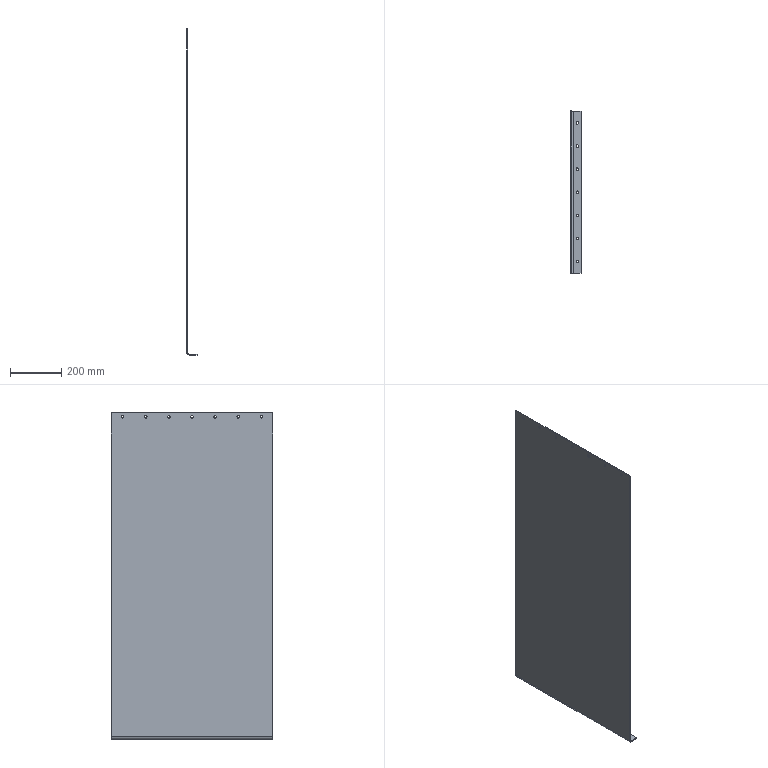Part | SolidWorks | features HoleWzd 2, LPattern 2, EdgeFlange 1, FlatPattern 1, ICE 1, SMBaseFlange 1, SheetMetal 1 | 1 solid | 42 faces | box 40 x 630 x 1270 mm | volume 3279151 mm3 | cylinder 30 | plane 12 | commonest cylinder face diameters 10 x29 18 x1
STEP:
#1=CARTESIAN_POINT('',(21.,40.,4.));
#2=VERTEX_POINT('',#1);
#3=CARTESIAN_POINT('',(21.,50.,4.));
#4=VERTEX_POINT('',#3);
#5=CARTESIAN_POINT('',(21.,45.,4.));
#6=DIRECTION('',(0.,0.,-1.));
#7=DIRECTION('',(0.,1.,0.));
#8=AXIS2_PLACEMENT_3D('',#5,#6,#7);
#9=CIRCLE('',#8,5.);
#10=EDGE_CURVE('',#2,#4,#9,.T.);
#11=ORIENTED_EDGE('',*,*,#10,.F.);
#12=CARTESIAN_POINT('',(21.,40.,0.));
#13=VERTEX_POINT('',#12);
#14=CARTESIAN_POINT('',(21.,40.,0.));
#15=DIRECTION('',(0.,0.,-1.));
#16=VECTOR('',#15,1000.);
#17=LINE('',#14,#16);
#18=EDGE_CURVE('',#2,#13,#17,.T.);
#19=ORIENTED_EDGE('',*,*,#18,.T.);
#20=CARTESIAN_POINT('',(21.,50.,0.));
#21=VERTEX_POINT('',#20);
#22=CARTESIAN_POINT('',(21.,45.,0.));
#23=DIRECTION('',(0.,0.,-1.));
#24=DIRECTION('',(0.,1.,0.));
#25=AXIS2_PLACEMENT_3D('',#22,#23,#24);
#26=CIRCLE('',#25,5.);
#27=EDGE_CURVE('',#13,#21,#26,.T.);
#28=ORIENTED_EDGE('',*,*,#27,.T.);
#29=CARTESIAN_POINT('',(21.,50.,0.));
#30=DIRECTION('',(0.,0.,-1.));
#31=VECTOR('',#30,1000.);
#32=LINE('',#29,#31);
#33=EDGE_CURVE('',#4,#21,#32,.T.);
#34=ORIENTED_EDGE('',*,*,#33,.F.);
#35=EDGE_LOOP('',(#11,#19,#28,#34));
#36=FACE_OUTER_BOUND('',#35,.T.);
#37=CARTESIAN_POINT('',(21.,45.,0.));
#38=DIRECTION('',(0.,0.,-1.));
#39=DIRECTION('',(0.,1.,0.));
#40=AXIS2_PLACEMENT_3D('',#37,#38,#39);
#41=CYLINDRICAL_SURFACE('',#40,5.);
#42=ADVANCED_FACE('',(#36),#41,.F.);
#43=CARTESIAN_POINT('',(21.,130.,4.));
#44=VERTEX_POINT('',#43);
#45=CARTESIAN_POINT('',(21.,140.,4.));
#46=VERTEX_POINT('',#45);
#47=CARTESIAN_POINT('',(21.,135.,4.));
#48=DIRECTION('',(0.,0.,-1.));
#49=DIRECTION('',(0.,1.,0.));
#50=AXIS2_PLACEMENT_3D('',#47,#48,#49);
#51=CIRCLE('',#50,5.);
#52=EDGE_CURVE('',#44,#46,#51,.T.);
#53=ORIENTED_EDGE('',*,*,#52,.F.);
#54=CARTESIAN_POINT('',(21.,130.,0.));
#55=VERTEX_POINT('',#54);
#56=CARTESIAN_POINT('',(21.,130.,0.));
#57=DIRECTION('',(0.,0.,-1.));
#58=VECTOR('',#57,1000.);
#59=LINE('',#56,#58);
#60=EDGE_CURVE('',#44,#55,#59,.T.);
#61=ORIENTED_EDGE('',*,*,#60,.T.);
#62=CARTESIAN_POINT('',(21.,140.,0.));
#63=VERTEX_POINT('',#62);
#64=CARTESIAN_POINT('',(21.,135.,0.));
#65=DIRECTION('',(0.,0.,-1.));
#66=DIRECTION('',(0.,1.,0.));
#67=AXIS2_PLACEMENT_3D('',#64,#65,#66);
#68=CIRCLE('',#67,5.);
#69=EDGE_CURVE('',#55,#63,#68,.T.);
#70=ORIENTED_EDGE('',*,*,#69,.T.);
#71=CARTESIAN_POINT('',(21.,140.,0.));
#72=DIRECTION('',(0.,0.,-1.));
#73=VECTOR('',#72,1000.);
#74=LINE('',#71,#73);
#75=EDGE_CURVE('',#46,#63,#74,.T.);
#76=ORIENTED_EDGE('',*,*,#75,.F.);
#77=EDGE_LOOP('',(#53,#61,#70,#76));
#78=FACE_OUTER_BOUND('',#77,.T.);
#79=CARTESIAN_POINT('',(21.,135.,0.));
#80=DIRECTION('',(0.,0.,-1.));
#81=DIRECTION('',(0.,1.,0.));
#82=AXIS2_PLACEMENT_3D('',#79,#80,#81);
#83=CYLINDRICAL_SURFACE('',#82,5.);
#84=ADVANCED_FACE('',(#78),#83,.F.);
#85=CARTESIAN_POINT('',(21.,220.,4.));
#86=VERTEX_POINT('',#85);
#87=CARTESIAN_POINT('',(21.,230.,4.));
#88=VERTEX_POINT('',#87);
#89=CARTESIAN_POINT('',(21.,225.,4.));
#90=DIRECTION('',(0.,0.,-1.));
#91=DIRECTION('',(0.,1.,0.));
#92=AXIS2_PLACEMENT_3D('',#89,#90,#91);
#93=CIRCLE('',#92,5.);
#94=EDGE_CURVE('',#86,#88,#93,.T.);
#95=ORIENTED_EDGE('',*,*,#94,.F.);
#96=CARTESIAN_POINT('',(21.,220.,0.));
#97=VERTEX_POINT('',#96);
#98=CARTESIAN_POINT('',(21.,220.,0.));
#99=DIRECTION('',(0.,0.,-1.));
#100=VECTOR('',#99,1000.);
#101=LINE('',#98,#100);
#102=EDGE_CURVE('',#86,#97,#101,.T.);
#103=ORIENTED_EDGE('',*,*,#102,.T.);
#104=CARTESIAN_POINT('',(21.,230.,0.));
#105=VERTEX_POINT('',#104);
#106=CARTESIAN_POINT('',(21.,225.,0.));
#107=DIRECTION('',(0.,0.,-1.));
#108=DIRECTION('',(0.,1.,0.));
#109=AXIS2_PLACEMENT_3D('',#106,#107,#108);
#110=CIRCLE('',#109,5.);
#111=EDGE_CURVE('',#97,#105,#110,.T.);
#112=ORIENTED_EDGE('',*,*,#111,.T.);
#113=CARTESIAN_POINT('',(21.,230.,0.));
#114=DIRECTION('',(0.,0.,-1.));
#115=VECTOR('',#114,1000.);
#116=LINE('',#113,#115);
#117=EDGE_CURVE('',#88,#105,#116,.T.);
#118=ORIENTED_EDGE('',*,*,#117,.F.);
#119=EDGE_LOOP('',(#95,#103,#112,#118));
#120=FACE_OUTER_BOUND('',#119,.T.);
#121=CARTESIAN_POINT('',(21.,225.,0.));
#122=DIRECTION('',(0.,0.,-1.));
#123=DIRECTION('',(0.,1.,0.));
#124=AXIS2_PLACEMENT_3D('',#121,#122,#123);
#125=CYLINDRICAL_SURFACE('',#124,5.);
#126=ADVANCED_FACE('',(#120),#125,.F.);
#127=CARTESIAN_POINT('',(21.,310.,4.));
#128=VERTEX_POINT('',#127);
#129=CARTESIAN_POINT('',(21.,320.,4.));
#130=VERTEX_POINT('',#129);
#131=CARTESIAN_POINT('',(21.,315.,4.));
#132=DIRECTION('',(0.,0.,-1.));
#133=DIRECTION('',(0.,1.,0.));
#134=AXIS2_PLACEMENT_3D('',#131,#132,#133);
#135=CIRCLE('',#134,5.);
#136=EDGE_CURVE('',#128,#130,#135,.T.);
#137=ORIENTED_EDGE('',*,*,#136,.F.);
#138=CARTESIAN_POINT('',(21.,310.,0.));
#139=VERTEX_POINT('',#138);
#140=CARTESIAN_POINT('',(21.,310.,0.));
#141=DIRECTION('',(0.,0.,-1.));
#142=VECTOR('',#141,1000.);
#143=LINE('',#140,#142);
#144=EDGE_CURVE('',#128,#139,#143,.T.);
#145=ORIENTED_EDGE('',*,*,#144,.T.);
#146=CARTESIAN_POINT('',(21.,320.,0.));
#147=VERTEX_POINT('',#146);
#148=CARTESIAN_POINT('',(21.,315.,0.));
#149=DIRECTION('',(0.,0.,-1.));
#150=DIRECTION('',(0.,1.,0.));
#151=AXIS2_PLACEMENT_3D('',#148,#149,#150);
#152=CIRCLE('',#151,5.);
#153=EDGE_CURVE('',#139,#147,#152,.T.);
#154=ORIENTED_EDGE('',*,*,#153,.T.);
#155=CARTESIAN_POINT('',(21.,320.,0.));
#156=DIRECTION('',(0.,0.,-1.));
#157=VECTOR('',#156,1000.);
#158=LINE('',#155,#157);
#159=EDGE_CURVE('',#130,#147,#158,.T.);
#160=ORIENTED_EDGE('',*,*,#159,.F.);
#161=EDGE_LOOP('',(#137,#145,#154,#160));
#162=FACE_OUTER_BOUND('',#161,.T.);
#163=CARTESIAN_POINT('',(21.,315.,0.));
#164=DIRECTION('',(0.,0.,-1.));
#165=DIRECTION('',(0.,1.,0.));
#166=AXIS2_PLACEMENT_3D('',#163,#164,#165);
#167=CYLINDRICAL_SURFACE('',#166,5.);
#168=ADVANCED_FACE('',(#162),#167,.F.);
#169=CARTESIAN_POINT('',(21.,400.,4.));
#170=VERTEX_POINT('',#169);
#171=CARTESIAN_POINT('',(21.,410.,4.));
#172=VERTEX_POINT('',#171);
#173=CARTESIAN_POINT('',(21.,405.,4.));
#174=DIRECTION('',(0.,0.,-1.));
#175=DIRECTION('',(0.,1.,0.));
#176=AXIS2_PLACEMENT_3D('',#173,#174,#175);
#177=CIRCLE('',#176,5.);
#178=EDGE_CURVE('',#170,#172,#177,.T.);
#179=ORIENTED_EDGE('',*,*,#178,.F.);
#180=CARTESIAN_POINT('',(21.,400.,0.));
#181=VERTEX_POINT('',#180);
#182=CARTESIAN_POINT('',(21.,400.,0.));
#183=DIRECTION('',(0.,0.,-1.));
#184=VECTOR('',#183,1000.);
#185=LINE('',#182,#184);
#186=EDGE_CURVE('',#170,#181,#185,.T.);
#187=ORIENTED_EDGE('',*,*,#186,.T.);
#188=CARTESIAN_POINT('',(21.,410.,0.));
#189=VERTEX_POINT('',#188);
#190=CARTESIAN_POINT('',(21.,405.,0.));
#191=DIRECTION('',(0.,0.,-1.));
#192=DIRECTION('',(0.,1.,0.));
#193=AXIS2_PLACEMENT_3D('',#190,#191,#192);
#194=CIRCLE('',#193,5.);
#195=EDGE_CURVE('',#181,#189,#194,.T.);
#196=ORIENTED_EDGE('',*,*,#195,.T.);
#197=CARTESIAN_POINT('',(21.,410.,0.));
#198=DIRECTION('',(0.,0.,-1.));
#199=VECTOR('',#198,1000.);
#200=LINE('',#197,#199);
#201=EDGE_CURVE('',#172,#189,#200,.T.);
#202=ORIENTED_EDGE('',*,*,#201,.F.);
#203=EDGE_LOOP('',(#179,#187,#196,#202));
#204=FACE_OUTER_BOUND('',#203,.T.);
#205=CARTESIAN_POINT('',(21.,405.,0.));
#206=DIRECTION('',(0.,0.,-1.));
#207=DIRECTION('',(0.,1.,0.));
#208=AXIS2_PLACEMENT_3D('',#205,#206,#207);
#209=CYLINDRICAL_SURFACE('',#208,5.);
#210=ADVANCED_FACE('',(#204),#209,.F.);
#211=CARTESIAN_POINT('',(21.,490.,4.));
#212=VERTEX_POINT('',#211);
#213=CARTESIAN_POINT('',(21.,500.,4.));
#214=VERTEX_POINT('',#213);
#215=CARTESIAN_POINT('',(21.,495.,4.));
#216=DIRECTION('',(0.,0.,-1.));
#217=DIRECTION('',(0.,1.,0.));
#218=AXIS2_PLACEMENT_3D('',#215,#216,#217);
#219=CIRCLE('',#218,5.);
#220=EDGE_CURVE('',#212,#214,#219,.T.);
#221=ORIENTED_EDGE('',*,*,#220,.F.);
#222=CARTESIAN_POINT('',(21.,490.,0.));
#223=VERTEX_POINT('',#222);
#224=CARTESIAN_POINT('',(21.,490.,0.));
#225=DIRECTION('',(0.,0.,-1.));
#226=VECTOR('',#225,1000.);
#227=LINE('',#224,#226);
#228=EDGE_CURVE('',#212,#223,#227,.T.);
#229=ORIENTED_EDGE('',*,*,#228,.T.);
#230=CARTESIAN_POINT('',(21.,500.,0.));
#231=VERTEX_POINT('',#230);
#232=CARTESIAN_POINT('',(21.,495.,0.));
#233=DIRECTION('',(0.,0.,-1.));
#234=DIRECTION('',(0.,1.,0.));
#235=AXIS2_PLACEMENT_3D('',#232,#233,#234);
#236=CIRCLE('',#235,5.);
#237=EDGE_CURVE('',#223,#231,#236,.T.);
#238=ORIENTED_EDGE('',*,*,#237,.T.);
#239=CARTESIAN_POINT('',(21.,500.,0.));
#240=DIRECTION('',(0.,0.,-1.));
#241=VECTOR('',#240,1000.);
#242=LINE('',#239,#241);
#243=EDGE_CURVE('',#214,#231,#242,.T.);
#244=ORIENTED_EDGE('',*,*,#243,.F.);
#245=EDGE_LOOP('',(#221,#229,#238,#244));
#246=FACE_OUTER_BOUND('',#245,.T.);
#247=CARTESIAN_POINT('',(21.,495.,0.));
#248=DIRECTION('',(0.,0.,-1.));
#249=DIRECTION('',(0.,1.,0.));
#250=AXIS2_PLACEMENT_3D('',#247,#248,#249);
#251=CYLINDRICAL_SURFACE('',#250,5.);
#252=ADVANCED_FACE('',(#246),#251,.F.);
#253=CARTESIAN_POINT('',(21.,580.,4.));
#254=VERTEX_POINT('',#253);
#255=CARTESIAN_POINT('',(21.,590.,4.));
#256=VERTEX_POINT('',#255);
#257=CARTESIAN_POINT('',(21.,585.,4.));
#258=DIRECTION('',(0.,0.,-1.));
#259=DIRECTION('',(0.,1.,0.));
#260=AXIS2_PLACEMENT_3D('',#257,#258,#259);
#261=CIRCLE('',#260,5.);
#262=EDGE_CURVE('',#254,#256,#261,.T.);
#263=ORIENTED_EDGE('',*,*,#262,.F.);
#264=CARTESIAN_POINT('',(21.,580.,0.));
#265=VERTEX_POINT('',#264);
#266=CARTESIAN_POINT('',(21.,580.,0.));
#267=DIRECTION('',(0.,0.,-1.));
#268=VECTOR('',#267,1000.);
#269=LINE('',#266,#268);
#270=EDGE_CURVE('',#254,#265,#269,.T.);
#271=ORIENTED_EDGE('',*,*,#270,.T.);
#272=CARTESIAN_POINT('',(21.,590.,0.));
#273=VERTEX_POINT('',#272);
#274=CARTESIAN_POINT('',(21.,585.,0.));
#275=DIRECTION('',(0.,0.,-1.));
#276=DIRECTION('',(0.,1.,0.));
#277=AXIS2_PLACEMENT_3D('',#274,#275,#276);
#278=CIRCLE('',#277,5.);
#279=EDGE_CURVE('',#265,#273,#278,.T.);
#280=ORIENTED_EDGE('',*,*,#279,.T.);
#281=CARTESIAN_POINT('',(21.,590.,0.));
#282=DIRECTION('',(0.,0.,-1.));
#283=VECTOR('',#282,1000.);
#284=LINE('',#281,#283);
#285=EDGE_CURVE('',#256,#273,#284,.T.);
#286=ORIENTED_EDGE('',*,*,#285,.F.);
#287=EDGE_LOOP('',(#263,#271,#280,#286));
#288=FACE_OUTER_BOUND('',#287,.T.);
#289=CARTESIAN_POINT('',(21.,585.,0.));
#290=DIRECTION('',(0.,0.,-1.));
#291=DIRECTION('',(0.,1.,0.));
#292=AXIS2_PLACEMENT_3D('',#289,#290,#291);
#293=CYLINDRICAL_SURFACE('',#292,5.);
#294=ADVANCED_FACE('',(#288),#293,.F.);
#295=CARTESIAN_POINT('',(-4.,45.,1260.));
#296=VERTEX_POINT('',#295);
#297=CARTESIAN_POINT('',(-4.,45.,1250.));
#298=VERTEX_POINT('',#297);
#299=CARTESIAN_POINT('',(-4.,45.,1255.));
#300=DIRECTION('',(1.,0.,0.));
#301=DIRECTION('',(0.,0.,-1.));
#302=AXIS2_PLACEMENT_3D('',#299,#300,#301);
#303=CIRCLE('',#302,5.);
#304=EDGE_CURVE('',#296,#298,#303,.T.);
#305=ORIENTED_EDGE('',*,*,#304,.F.);
#306=CARTESIAN_POINT('',(0.,45.,1260.));
#307=VERTEX_POINT('',#306);
#308=CARTESIAN_POINT('',(0.,45.,1260.));
#309=DIRECTION('',(1.,0.,0.));
#310=VECTOR('',#309,1000.);
#311=LINE('',#308,#310);
#312=EDGE_CURVE('',#296,#307,#311,.T.);
#313=ORIENTED_EDGE('',*,*,#312,.T.);
#314=CARTESIAN_POINT('',(0.,45.,1250.));
#315=VERTEX_POINT('',#314);
#316=CARTESIAN_POINT('',(0.,45.,1255.));
#317=DIRECTION('',(1.,0.,0.));
#318=DIRECTION('',(0.,0.,-1.));
#319=AXIS2_PLACEMENT_3D('',#316,#317,#318);
#320=CIRCLE('',#319,5.);
#321=EDGE_CURVE('',#307,#315,#320,.T.);
#322=ORIENTED_EDGE('',*,*,#321,.T.);
#323=CARTESIAN_POINT('',(0.,45.,1250.));
#324=DIRECTION('',(1.,0.,0.));
#325=VECTOR('',#324,1000.);
#326=LINE('',#323,#325);
#327=EDGE_CURVE('',#298,#315,#326,.T.);
#328=ORIENTED_EDGE('',*,*,#327,.F.);
#329=EDGE_LOOP('',(#305,#313,#322,#328));
#330=FACE_OUTER_BOUND('',#329,.T.);
#331=CARTESIAN_POINT('',(0.,45.,1255.));
#332=DIRECTION('',(1.,0.,0.));
#333=DIRECTION('',(0.,0.,-1.));
#334=AXIS2_PLACEMENT_3D('',#331,#332,#333);
#335=CYLINDRICAL_SURFACE('',#334,5.);
#336=ADVANCED_FACE('',(#330),#335,.F.);
#337=CARTESIAN_POINT('',(-4.,135.,1260.));
#338=VERTEX_POINT('',#337);
#339=CARTESIAN_POINT('',(-4.,135.,1250.));
#340=VERTEX_POINT('',#339);
#341=CARTESIAN_POINT('',(-4.,135.,1255.));
#342=DIRECTION('',(1.,0.,0.));
#343=DIRECTION('',(0.,0.,-1.));
#344=AXIS2_PLACEMENT_3D('',#341,#342,#343);
#345=CIRCLE('',#344,5.);
#346=EDGE_CURVE('',#338,#340,#345,.T.);
#347=ORIENTED_EDGE('',*,*,#346,.F.);
#348=CARTESIAN_POINT('',(0.,135.,1260.));
#349=VERTEX_POINT('',#348);
#350=CARTESIAN_POINT('',(0.,135.,1260.));
#351=DIRECTION('',(1.,0.,0.));
#352=VECTOR('',#351,1000.);
#353=LINE('',#350,#352);
#354=EDGE_CURVE('',#338,#349,#353,.T.);
#355=ORIENTED_EDGE('',*,*,#354,.T.);
#356=CARTESIAN_POINT('',(0.,135.,1250.));
#357=VERTEX_POINT('',#356);
#358=CARTESIAN_POINT('',(0.,135.,1255.));
#359=DIRECTION('',(1.,0.,0.));
#360=DIRECTION('',(0.,0.,-1.));
#361=AXIS2_PLACEMENT_3D('',#358,#359,#360);
#362=CIRCLE('',#361,5.);
#363=EDGE_CURVE('',#349,#357,#362,.T.);
#364=ORIENTED_EDGE('',*,*,#363,.T.);
#365=CARTESIAN_POINT('',(0.,135.,1250.));
#366=DIRECTION('',(1.,0.,0.));
#367=VECTOR('',#366,1000.);
#368=LINE('',#365,#367);
#369=EDGE_CURVE('',#340,#357,#368,.T.);
#370=ORIENTED_EDGE('',*,*,#369,.F.);
#371=EDGE_LOOP('',(#347,#355,#364,#370));
#372=FACE_OUTER_BOUND('',#371,.T.);
#373=CARTESIAN_POINT('',(0.,135.,1255.));
#374=DIRECTION('',(1.,0.,0.));
#375=DIRECTION('',(0.,0.,-1.));
#376=AXIS2_PLACEMENT_3D('',#373,#374,#375);
#377=CYLINDRICAL_SURFACE('',#376,5.);
#378=ADVANCED_FACE('',(#372),#377,.F.);
#379=CARTESIAN_POINT('',(-4.,225.,1260.));
#380=VERTEX_POINT('',#379);
#381=CARTESIAN_POINT('',(-4.,225.,1250.));
#382=VERTEX_POINT('',#381);
#383=CARTESIAN_POINT('',(-4.,225.,1255.));
#384=DIRECTION('',(1.,0.,0.));
#385=DIRECTION('',(0.,0.,-1.));
#386=AXIS2_PLACEMENT_3D('',#383,#384,#385);
#387=CIRCLE('',#386,5.);
#388=EDGE_CURVE('',#380,#382,#387,.T.);
#389=ORIENTED_EDGE('',*,*,#388,.F.);
#390=CARTESIAN_POINT('',(0.,225.,1260.));
#391=VERTEX_POINT('',#390);
#392=CARTESIAN_POINT('',(0.,225.,1260.));
#393=DIRECTION('',(1.,0.,0.));
#394=VECTOR('',#393,1000.);
#395=LINE('',#392,#394);
#396=EDGE_CURVE('',#380,#391,#395,.T.);
#397=ORIENTED_EDGE('',*,*,#396,.T.);
#398=CARTESIAN_POINT('',(0.,225.,1250.));
#399=VERTEX_POINT('',#398);
#400=CARTESIAN_POINT('',(0.,225.,1255.));
#401=DIRECTION('',(1.,0.,0.));
#402=DIRECTION('',(0.,0.,-1.));
#403=AXIS2_PLACEMENT_3D('',#400,#401,#402);
#404=CIRCLE('',#403,5.);
#405=EDGE_CURVE('',#391,#399,#404,.T.);
#406=ORIENTED_EDGE('',*,*,#405,.T.);
#407=CARTESIAN_POINT('',(0.,225.,1250.));
#408=DIRECTION('',(1.,0.,0.));
#409=VECTOR('',#408,1000.);
#410=LINE('',#407,#409);
#411=EDGE_CURVE('',#382,#399,#410,.T.);
#412=ORIENTED_EDGE('',*,*,#411,.F.);
#413=EDGE_LOOP('',(#389,#397,#406,#412));
#414=FACE_OUTER_BOUND('',#413,.T.);
#415=CARTESIAN_POINT('',(0.,225.,1255.));
#416=DIRECTION('',(1.,0.,0.));
#417=DIRECTION('',(0.,0.,-1.));
#418=AXIS2_PLACEMENT_3D('',#415,#416,#417);
#419=CYLINDRICAL_SURFACE('',#418,5.);
#420=ADVANCED_FACE('',(#414),#419,.F.);
#421=CARTESIAN_POINT('',(-4.,315.,1260.));
#422=VERTEX_POINT('',#421);
#423=CARTESIAN_POINT('',(-4.,315.,1250.));
#424=VERTEX_POINT('',#423);
#425=CARTESIAN_POINT('',(-4.,315.,1255.));
#426=DIRECTION('',(1.,0.,0.));
#427=DIRECTION('',(0.,0.,-1.));
#428=AXIS2_PLACEMENT_3D('',#425,#426,#427);
#429=CIRCLE('',#428,5.);
#430=EDGE_CURVE('',#422,#424,#429,.T.);
#431=ORIENTED_EDGE('',*,*,#430,.F.);
#432=CARTESIAN_POINT('',(0.,315.,1260.));
#433=VERTEX_POINT('',#432);
#434=CARTESIAN_POINT('',(0.,315.,1260.));
#435=DIRECTION('',(1.,0.,0.));
#436=VECTOR('',#435,1000.);
#437=LINE('',#434,#436);
#438=EDGE_CURVE('',#422,#433,#437,.T.);
#439=ORIENTED_EDGE('',*,*,#438,.T.);
#440=CARTESIAN_POINT('',(0.,315.,1250.));
#441=VERTEX_POINT('',#440);
#442=CARTESIAN_POINT('',(0.,315.,1255.));
#443=DIRECTION('',(1.,0.,0.));
#444=DIRECTION('',(0.,0.,-1.));
#445=AXIS2_PLACEMENT_3D('',#442,#443,#444);
#446=CIRCLE('',#445,5.);
#447=EDGE_CURVE('',#433,#441,#446,.T.);
#448=ORIENTED_EDGE('',*,*,#447,.T.);
#449=CARTESIAN_POINT('',(0.,315.,1250.));
#450=DIRECTION('',(1.,0.,0.));
#451=VECTOR('',#450,1000.);
#452=LINE('',#449,#451);
#453=EDGE_CURVE('',#424,#441,#452,.T.);
#454=ORIENTED_EDGE('',*,*,#453,.F.);
#455=EDGE_LOOP('',(#431,#439,#448,#454));
#456=FACE_OUTER_BOUND('',#455,.T.);
#457=CARTESIAN_POINT('',(0.,315.,1255.));
#458=DIRECTION('',(1.,0.,0.));
#459=DIRECTION('',(0.,0.,-1.));
#460=AXIS2_PLACEMENT_3D('',#457,#458,#459);
#461=CYLINDRICAL_SURFACE('',#460,5.);
#462=ADVANCED_FACE('',(#456),#461,.F.);
#463=CARTESIAN_POINT('',(-4.,405.,1260.));
#464=VERTEX_POINT('',#463);
#465=CARTESIAN_POINT('',(-4.,405.,1250.));
#466=VERTEX_POINT('',#465);
#467=CARTESIAN_POINT('',(-4.,405.,1255.));
#468=DIRECTION('',(1.,0.,0.));
#469=DIRECTION('',(0.,0.,-1.));
#470=AXIS2_PLACEMENT_3D('',#467,#468,#469);
#471=CIRCLE('',#470,5.);
#472=EDGE_CURVE('',#464,#466,#471,.T.);
#473=ORIENTED_EDGE('',*,*,#472,.F.);
#474=CARTESIAN_POINT('',(0.,405.,1260.));
#475=VERTEX_POINT('',#474);
#476=CARTESIAN_POINT('',(0.,405.,1260.));
#477=DIRECTION('',(1.,0.,0.));
#478=VECTOR('',#477,1000.);
#479=LINE('',#476,#478);
#480=EDGE_CURVE('',#464,#475,#479,.T.);
#481=ORIENTED_EDGE('',*,*,#480,.T.);
#482=CARTESIAN_POINT('',(0.,405.,1250.));
#483=VERTEX_POINT('',#482);
#484=CARTESIAN_POINT('',(0.,405.,1255.));
#485=DIRECTION('',(1.,0.,0.));
#486=DIRECTION('',(0.,0.,-1.));
#487=AXIS2_PLACEMENT_3D('',#484,#485,#486);
#488=CIRCLE('',#487,5.);
#489=EDGE_CURVE('',#475,#483,#488,.T.);
#490=ORIENTED_EDGE('',*,*,#489,.T.);
#491=CARTESIAN_POINT('',(0.,405.,1250.));
#492=DIRECTION('',(1.,0.,0.));
#493=VECTOR('',#492,1000.);
#494=LINE('',#491,#493);
#495=EDGE_CURVE('',#466,#483,#494,.T.);
#496=ORIENTED_EDGE('',*,*,#495,.F.);
#497=EDGE_LOOP('',(#473,#481,#490,#496));
#498=FACE_OUTER_BOUND('',#497,.T.);
#499=CARTESIAN_POINT('',(0.,405.,1255.));
#500=DIRECTION('',(1.,0.,0.));
#501=DIRECTION('',(0.,0.,-1.));
#502=AXIS2_PLACEMENT_3D('',#499,#500,#501);
#503=CYLINDRICAL_SURFACE('',#502,5.);
#504=ADVANCED_FACE('',(#498),#503,.F.);
#505=CARTESIAN_POINT('',(-4.,495.,1260.));
#506=VERTEX_POINT('',#505);
#507=CARTESIAN_POINT('',(-4.,495.,1250.));
#508=VERTEX_POINT('',#507);
#509=CARTESIAN_POINT('',(-4.,495.,1255.));
#510=DIRECTION('',(1.,0.,0.));
#511=DIRECTION('',(0.,0.,-1.));
#512=AXIS2_PLACEMENT_3D('',#509,#510,#511);
#513=CIRCLE('',#512,5.);
#514=EDGE_CURVE('',#506,#508,#513,.T.);
#515=ORIENTED_EDGE('',*,*,#514,.F.);
#516=CARTESIAN_POINT('',(0.,495.,1260.));
#517=VERTEX_POINT('',#516);
#518=CARTESIAN_POINT('',(0.,495.,1260.));
#519=DIRECTION('',(1.,0.,0.));
#520=VECTOR('',#519,1000.);
#521=LINE('',#518,#520);
#522=EDGE_CURVE('',#506,#517,#521,.T.);
#523=ORIENTED_EDGE('',*,*,#522,.T.);
#524=CARTESIAN_POINT('',(0.,495.,1250.));
#525=VERTEX_POINT('',#524);
#526=CARTESIAN_POINT('',(0.,495.,1255.));
#527=DIRECTION('',(1.,0.,0.));
#528=DIRECTION('',(0.,0.,-1.));
#529=AXIS2_PLACEMENT_3D('',#526,#527,#528);
#530=CIRCLE('',#529,5.);
#531=EDGE_CURVE('',#517,#525,#530,.T.);
#532=ORIENTED_EDGE('',*,*,#531,.T.);
#533=CARTESIAN_POINT('',(0.,495.,1250.));
#534=DIRECTION('',(1.,0.,0.));
#535=VECTOR('',#534,1000.);
#536=LINE('',#533,#535);
#537=EDGE_CURVE('',#508,#525,#536,.T.);
#538=ORIENTED_EDGE('',*,*,#537,.F.);
#539=EDGE_LOOP('',(#515,#523,#532,#538));
#540=FACE_OUTER_BOUND('',#539,.T.);
#541=CARTESIAN_POINT('',(0.,495.,1255.));
#542=DIRECTION('',(1.,0.,0.));
#543=DIRECTION('',(0.,0.,-1.));
#544=AXIS2_PLACEMENT_3D('',#541,#542,#543);
#545=CYLINDRICAL_SURFACE('',#544,5.);
#546=ADVANCED_FACE('',(#540),#545,.F.);
#547=CARTESIAN_POINT('',(-4.,585.,1260.));
#548=VERTEX_POINT('',#547);
#549=CARTESIAN_POINT('',(-4.,585.,1250.));
#550=VERTEX_POINT('',#549);
#551=CARTESIAN_POINT('',(-4.,585.,1255.));
#552=DIRECTION('',(1.,0.,0.));
#553=DIRECTION('',(0.,0.,-1.));
#554=AXIS2_PLACEMENT_3D('',#551,#552,#553);
#555=CIRCLE('',#554,5.);
#556=EDGE_CURVE('',#548,#550,#555,.T.);
#557=ORIENTED_EDGE('',*,*,#556,.F.);
#558=CARTESIAN_POINT('',(0.,585.,1260.));
#559=VERTEX_POINT('',#558);
#560=CARTESIAN_POINT('',(0.,585.,1260.));
#561=DIRECTION('',(1.,0.,0.));
#562=VECTOR('',#561,1000.);
#563=LINE('',#560,#562);
#564=EDGE_CURVE('',#548,#559,#563,.T.);
#565=ORIENTED_EDGE('',*,*,#564,.T.);
#566=CARTESIAN_POINT('',(0.,585.,1250.));
#567=VERTEX_POINT('',#566);
#568=CARTESIAN_POINT('',(0.,585.,1255.));
#569=DIRECTION('',(1.,0.,0.));
#570=DIRECTION('',(0.,0.,-1.));
#571=AXIS2_PLACEMENT_3D('',#568,#569,#570);
#572=CIRCLE('',#571,5.);
#573=EDGE_CURVE('',#559,#567,#572,.T.);
#574=ORIENTED_EDGE('',*,*,#573,.T.);
#575=CARTESIAN_POINT('',(0.,585.,1250.));
#576=DIRECTION('',(1.,0.,0.));
#577=VECTOR('',#576,1000.);
#578=LINE('',#575,#577);
#579=EDGE_CURVE('',#550,#567,#578,.T.);
#580=ORIENTED_EDGE('',*,*,#579,.F.);
#581=EDGE_LOOP('',(#557,#565,#574,#580));
#582=FACE_OUTER_BOUND('',#581,.T.);
#583=CARTESIAN_POINT('',(0.,585.,1255.));
#584=DIRECTION('',(1.,0.,0.));
#585=DIRECTION('',(0.,0.,-1.));
#586=AXIS2_PLACEMENT_3D('',#583,#584,#585);
#587=CYLINDRICAL_SURFACE('',#586,5.);
#588=ADVANCED_FACE('',(#582),#587,.F.);
#589=CARTESIAN_POINT('',(0.,630.,9.));
#590=VERTEX_POINT('',#589);
#591=CARTESIAN_POINT('',(0.,630.,1270.));
#592=VERTEX_POINT('',#591);
#593=CARTESIAN_POINT('',(0.,630.,1270.));
#594=DIRECTION('',(0.,0.,1.));
#595=VECTOR('',#594,1000.);
#596=LINE('',#593,#595);
#597=EDGE_CURVE('',#590,#592,#596,.T.);
#598=ORIENTED_EDGE('',*,*,#597,.F.);
#599=CARTESIAN_POINT('',(-4.,630.,9.));
#600=VERTEX_POINT('',#599);
#601=CARTESIAN_POINT('',(0.,630.,9.));
#602=DIRECTION('',(-1.,0.,0.));
#603=VECTOR('',#602,1000.);
#604=LINE('',#601,#603);
#605=EDGE_CURVE('',#590,#600,#604,.T.);
#606=ORIENTED_EDGE('',*,*,#605,.T.);
#607=CARTESIAN_POINT('',(-4.,630.,1270.));
#608=VERTEX_POINT('',#607);
#609=CARTESIAN_POINT('',(-4.,630.,1270.));
#610=DIRECTION('',(0.,0.,1.));
#611=VECTOR('',#610,1000.);
#612=LINE('',#609,#611);
#613=EDGE_CURVE('',#600,#608,#612,.T.);
#614=ORIENTED_EDGE('',*,*,#613,.T.);
#615=CARTESIAN_POINT('',(-4.,630.,1270.));
#616=DIRECTION('',(1.,0.,0.));
#617=VECTOR('',#616,1000.);
#618=LINE('',#615,#617);
#619=EDGE_CURVE('',#608,#592,#618,.T.);
#620=ORIENTED_EDGE('',*,*,#619,.T.);
#621=EDGE_LOOP('',(#598,#606,#614,#620));
#622=FACE_OUTER_BOUND('',#621,.T.);
#623=CARTESIAN_POINT('',(-4.,630.,1270.));
#624=DIRECTION('',(0.,1.,0.));
#625=DIRECTION('',(0.,0.,1.));
#626=AXIS2_PLACEMENT_3D('',#623,#624,#625);
#627=PLANE('',#626);
#628=ADVANCED_FACE('',(#622),#627,.T.);
#629=CARTESIAN_POINT('',(-4.,495.,1255.));
#630=DIRECTION('',(1.,0.,0.));
#631=DIRECTION('',(0.,0.,-1.));
#632=AXIS2_PLACEMENT_3D('',#629,#630,#631);
#633=CIRCLE('',#632,5.);
#634=EDGE_CURVE('',#508,#506,#633,.T.);
#635=ORIENTED_EDGE('',*,*,#634,.T.);
#636=ORIENTED_EDGE('',*,*,#514,.T.);
#637=EDGE_LOOP('',(#635,#636));
#638=FACE_BOUND('',#637,.T.);
#639=CARTESIAN_POINT('',(-4.,585.,1255.));
#640=DIRECTION('',(1.,0.,0.));
#641=DIRECTION('',(0.,0.,-1.));
#642=AXIS2_PLACEMENT_3D('',#639,#640,#641);
#643=CIRCLE('',#642,5.);
#644=EDGE_CURVE('',#550,#548,#643,.T.);
#645=ORIENTED_EDGE('',*,*,#644,.T.);
#646=ORIENTED_EDGE('',*,*,#556,.T.);
#647=EDGE_LOOP('',(#645,#646));
#648=FACE_BOUND('',#647,.T.);
#649=CARTESIAN_POINT('',(-4.,0.,9.));
#650=VERTEX_POINT('',#649);
#651=CARTESIAN_POINT('',(-4.,630.,9.));
#652=DIRECTION('',(0.,-1.,0.));
#653=VECTOR('',#652,1000.);
#654=LINE('',#651,#653);
#655=EDGE_CURVE('',#600,#650,#654,.T.);
#656=ORIENTED_EDGE('',*,*,#655,.T.);
#657=CARTESIAN_POINT('',(-4.,0.,1270.));
#658=VERTEX_POINT('',#657);
#659=CARTESIAN_POINT('',(-4.,0.,1270.));
#660=DIRECTION('',(0.,0.,-1.));
#661=VECTOR('',#660,1000.);
#662=LINE('',#659,#661);
#663=EDGE_CURVE('',#658,#650,#662,.T.);
#664=ORIENTED_EDGE('',*,*,#663,.F.);
#665=CARTESIAN_POINT('',(-4.,630.,1270.));
#666=DIRECTION('',(0.,-1.,0.));
#667=VECTOR('',#666,1000.);
#668=LINE('',#665,#667);
#669=EDGE_CURVE('',#608,#658,#668,.T.);
#670=ORIENTED_EDGE('',*,*,#669,.F.);
#671=ORIENTED_EDGE('',*,*,#613,.F.);
#672=EDGE_LOOP('',(#656,#664,#670,#671));
#673=FACE_OUTER_BOUND('',#672,.T.);
#674=CARTESIAN_POINT('',(-4.,405.,1255.));
#675=DIRECTION('',(1.,0.,0.));
#676=DIRECTION('',(0.,0.,-1.));
#677=AXIS2_PLACEMENT_3D('',#674,#675,#676);
#678=CIRCLE('',#677,5.);
#679=EDGE_CURVE('',#466,#464,#678,.T.);
#680=ORIENTED_EDGE('',*,*,#679,.T.);
#681=ORIENTED_EDGE('',*,*,#472,.T.);
#682=EDGE_LOOP('',(#680,#681));
#683=FACE_BOUND('',#682,.T.);
#684=CARTESIAN_POINT('',(-4.,315.,1255.));
#685=DIRECTION('',(1.,0.,0.));
#686=DIRECTION('',(0.,0.,-1.));
#687=AXIS2_PLACEMENT_3D('',#684,#685,#686);
#688=CIRCLE('',#687,5.);
#689=EDGE_CURVE('',#424,#422,#688,.T.);
#690=ORIENTED_EDGE('',*,*,#689,.T.);
#691=ORIENTED_EDGE('',*,*,#430,.T.);
#692=EDGE_LOOP('',(#690,#691));
#693=FACE_BOUND('',#692,.T.);
#694=CARTESIAN_POINT('',(-4.,225.,1255.));
#695=DIRECTION('',(1.,0.,0.));
#696=DIRECTION('',(0.,0.,-1.));
#697=AXIS2_PLACEMENT_3D('',#694,#695,#696);
#698=CIRCLE('',#697,5.);
#699=EDGE_CURVE('',#382,#380,#698,.T.);
#700=ORIENTED_EDGE('',*,*,#699,.T.);
#701=ORIENTED_EDGE('',*,*,#388,.T.);
#702=EDGE_LOOP('',(#700,#701));
#703=FACE_BOUND('',#702,.T.);
#704=CARTESIAN_POINT('',(-4.,135.,1255.));
#705=DIRECTION('',(1.,0.,0.));
#706=DIRECTION('',(0.,0.,-1.));
#707=AXIS2_PLACEMENT_3D('',#704,#705,#706);
#708=CIRCLE('',#707,5.);
#709=EDGE_CURVE('',#340,#338,#708,.T.);
#710=ORIENTED_EDGE('',*,*,#709,.T.);
#711=ORIENTED_EDGE('',*,*,#346,.T.);
#712=EDGE_LOOP('',(#710,#711));
#713=FACE_BOUND('',#712,.T.);
#714=CARTESIAN_POINT('',(-4.,45.,1255.));
#715=DIRECTION('',(1.,0.,0.));
#716=DIRECTION('',(0.,0.,-1.));
#717=AXIS2_PLACEMENT_3D('',#714,#715,#716);
#718=CIRCLE('',#717,5.);
#719=EDGE_CURVE('',#298,#296,#718,.T.);
#720=ORIENTED_EDGE('',*,*,#719,.T.);
#721=ORIENTED_EDGE('',*,*,#304,.T.);
#722=EDGE_LOOP('',(#720,#721));
#723=FACE_BOUND('',#722,.T.);
#724=CARTESIAN_POINT('',(-4.,0.,1270.));
#725=DIRECTION('',(1.,0.,0.));
#726=DIRECTION('',(0.,0.,-1.));
#727=AXIS2_PLACEMENT_3D('',#724,#725,#726);
#728=PLANE('',#727);
#729=ADVANCED_FACE('',(#638,#648,#673,#683,#693,#703,#713,#723),#728,.F.);
#730=CARTESIAN_POINT('',(0.,495.,1255.));
#731=DIRECTION('',(1.,0.,0.));
#732=DIRECTION('',(0.,0.,-1.));
#733=AXIS2_PLACEMENT_3D('',#730,#731,#732);
#734=CIRCLE('',#733,5.);
#735=EDGE_CURVE('',#525,#517,#734,.T.);
#736=ORIENTED_EDGE('',*,*,#735,.F.);
#737=ORIENTED_EDGE('',*,*,#531,.F.);
#738=EDGE_LOOP('',(#736,#737));
#739=FACE_BOUND('',#738,.T.);
#740=CARTESIAN_POINT('',(0.,585.,1255.));
#741=DIRECTION('',(1.,0.,0.));
#742=DIRECTION('',(0.,0.,-1.));
#743=AXIS2_PLACEMENT_3D('',#740,#741,#742);
#744=CIRCLE('',#743,5.);
#745=EDGE_CURVE('',#567,#559,#744,.T.);
#746=ORIENTED_EDGE('',*,*,#745,.F.);
#747=ORIENTED_EDGE('',*,*,#573,.F.);
#748=EDGE_LOOP('',(#746,#747));
#749=FACE_BOUND('',#748,.T.);
#750=CARTESIAN_POINT('',(0.,0.,1270.));
#751=VERTEX_POINT('',#750);
#752=CARTESIAN_POINT('',(0.,0.,9.));
#753=VERTEX_POINT('',#752);
#754=CARTESIAN_POINT('',(0.,0.,1270.));
#755=DIRECTION('',(0.,0.,-1.));
#756=VECTOR('',#755,1000.);
#757=LINE('',#754,#756);
#758=EDGE_CURVE('',#751,#753,#757,.T.);
#759=ORIENTED_EDGE('',*,*,#758,.T.);
#760=CARTESIAN_POINT('',(0.,630.,9.));
#761=DIRECTION('',(0.,-1.,0.));
#762=VECTOR('',#761,1000.);
#763=LINE('',#760,#762);
#764=EDGE_CURVE('',#590,#753,#763,.T.);
#765=ORIENTED_EDGE('',*,*,#764,.F.);
#766=ORIENTED_EDGE('',*,*,#597,.T.);
#767=CARTESIAN_POINT('',(0.,630.,1270.));
#768=DIRECTION('',(0.,-1.,0.));
#769=VECTOR('',#768,1000.);
#770=LINE('',#767,#769);
#771=EDGE_CURVE('',#592,#751,#770,.T.);
#772=ORIENTED_EDGE('',*,*,#771,.T.);
#773=EDGE_LOOP('',(#759,#765,#766,#772));
#774=FACE_OUTER_BOUND('',#773,.T.);
#775=CARTESIAN_POINT('',(0.,405.,1255.));
#776=DIRECTION('',(1.,0.,0.));
#777=DIRECTION('',(0.,0.,-1.));
#778=AXIS2_PLACEMENT_3D('',#775,#776,#777);
#779=CIRCLE('',#778,5.);
#780=EDGE_CURVE('',#483,#475,#779,.T.);
#781=ORIENTED_EDGE('',*,*,#780,.F.);
#782=ORIENTED_EDGE('',*,*,#489,.F.);
#783=EDGE_LOOP('',(#781,#782));
#784=FACE_BOUND('',#783,.T.);
#785=CARTESIAN_POINT('',(0.,315.,1255.));
#786=DIRECTION('',(1.,0.,0.));
#787=DIRECTION('',(0.,0.,-1.));
#788=AXIS2_PLACEMENT_3D('',#785,#786,#787);
#789=CIRCLE('',#788,5.);
#790=EDGE_CURVE('',#441,#433,#789,.T.);
#791=ORIENTED_EDGE('',*,*,#790,.F.);
#792=ORIENTED_EDGE('',*,*,#447,.F.);
#793=EDGE_LOOP('',(#791,#792));
#794=FACE_BOUND('',#793,.T.);
#795=CARTESIAN_POINT('',(0.,225.,1255.));
#796=DIRECTION('',(1.,0.,0.));
#797=DIRECTION('',(0.,0.,-1.));
#798=AXIS2_PLACEMENT_3D('',#795,#796,#797);
#799=CIRCLE('',#798,5.);
#800=EDGE_CURVE('',#399,#391,#799,.T.);
#801=ORIENTED_EDGE('',*,*,#800,.F.);
#802=ORIENTED_EDGE('',*,*,#405,.F.);
#803=EDGE_LOOP('',(#801,#802));
#804=FACE_BOUND('',#803,.T.);
#805=CARTESIAN_POINT('',(0.,135.,1255.));
#806=DIRECTION('',(1.,0.,0.));
#807=DIRECTION('',(0.,0.,-1.));
#808=AXIS2_PLACEMENT_3D('',#805,#806,#807);
#809=CIRCLE('',#808,5.);
#810=EDGE_CURVE('',#357,#349,#809,.T.);
#811=ORIENTED_EDGE('',*,*,#810,.F.);
#812=ORIENTED_EDGE('',*,*,#363,.F.);
#813=EDGE_LOOP('',(#811,#812));
#814=FACE_BOUND('',#813,.T.);
#815=CARTESIAN_POINT('',(0.,45.,1255.));
#816=DIRECTION('',(1.,0.,0.));
#817=DIRECTION('',(0.,0.,-1.));
#818=AXIS2_PLACEMENT_3D('',#815,#816,#817);
#819=CIRCLE('',#818,5.);
#820=EDGE_CURVE('',#315,#307,#819,.T.);
#821=ORIENTED_EDGE('',*,*,#820,.F.);
#822=ORIENTED_EDGE('',*,*,#321,.F.);
#823=EDGE_LOOP('',(#821,#822));
#824=FACE_BOUND('',#823,.T.);
#825=CARTESIAN_POINT('',(0.,0.,1270.));
#826=DIRECTION('',(1.,0.,0.));
#827=DIRECTION('',(0.,0.,-1.));
#828=AXIS2_PLACEMENT_3D('',#825,#826,#827);
#829=PLANE('',#828);
#830=ADVANCED_FACE('',(#739,#749,#774,#784,#794,#804,#814,#824),#829,.T.);
#831=ORIENTED_EDGE('',*,*,#771,.F.);
#832=ORIENTED_EDGE('',*,*,#619,.F.);
#833=ORIENTED_EDGE('',*,*,#669,.T.);
#834=CARTESIAN_POINT('',(-4.,0.,1270.));
#835=DIRECTION('',(1.,0.,0.));
#836=VECTOR('',#835,1000.);
#837=LINE('',#834,#836);
#838=EDGE_CURVE('',#658,#751,#837,.T.);
#839=ORIENTED_EDGE('',*,*,#838,.T.);
#840=EDGE_LOOP('',(#831,#832,#833,#839));
#841=FACE_OUTER_BOUND('',#840,.T.);
#842=CARTESIAN_POINT('',(-4.,630.,1270.));
#843=DIRECTION('',(0.,0.,1.));
#844=DIRECTION('',(1.,0.,0.));
#845=AXIS2_PLACEMENT_3D('',#842,#843,#844);
#846=PLANE('',#845);
#847=ADVANCED_FACE('',(#841),#846,.T.);
#848=CARTESIAN_POINT('',(0.,0.,9.));
#849=DIRECTION('',(-1.,0.,0.));
#850=VECTOR('',#849,1000.);
#851=LINE('',#848,#850);
#852=EDGE_CURVE('',#753,#650,#851,.T.);
#853=ORIENTED_EDGE('',*,*,#852,.F.);
#854=ORIENTED_EDGE('',*,*,#758,.F.);
#855=ORIENTED_EDGE('',*,*,#838,.F.);
#856=ORIENTED_EDGE('',*,*,#663,.T.);
#857=EDGE_LOOP('',(#853,#854,#855,#856));
#858=FACE_OUTER_BOUND('',#857,.T.);
#859=CARTESIAN_POINT('',(-4.,0.,1270.));
#860=DIRECTION('',(0.,-1.,0.));
#861=DIRECTION('',(0.,0.,-1.));
#862=AXIS2_PLACEMENT_3D('',#859,#860,#861);
#863=PLANE('',#862);
#864=ADVANCED_FACE('',(#858),#863,.T.);
#865=CARTESIAN_POINT('',(5.,0.,4.));
#866=VERTEX_POINT('',#865);
#867=CARTESIAN_POINT('',(5.,0.,0.));
#868=VERTEX_POINT('',#867);
#869=CARTESIAN_POINT('',(5.,0.,0.));
#870=DIRECTION('',(0.,0.,-1.));
#871=VECTOR('',#870,1000.);
#872=LINE('',#869,#871);
#873=EDGE_CURVE('',#866,#868,#872,.T.);
#874=ORIENTED_EDGE('',*,*,#873,.F.);
#875=CARTESIAN_POINT('',(5.,0.,9.));
#876=DIRECTION('',(0.,-1.,0.));
#877=DIRECTION('',(0.,0.,1.));
#878=AXIS2_PLACEMENT_3D('',#875,#876,#877);
#879=CIRCLE('',#878,5.);
#880=EDGE_CURVE('',#753,#866,#879,.T.);
#881=ORIENTED_EDGE('',*,*,#880,.F.);
#882=ORIENTED_EDGE('',*,*,#852,.T.);
#883=CARTESIAN_POINT('',(5.,0.,9.));
#884=DIRECTION('',(0.,-1.,0.));
#885=DIRECTION('',(0.,0.,1.));
#886=AXIS2_PLACEMENT_3D('',#883,#884,#885);
#887=CIRCLE('',#886,9.);
#888=EDGE_CURVE('',#650,#868,#887,.T.);
#889=ORIENTED_EDGE('',*,*,#888,.T.);
#890=EDGE_LOOP('',(#874,#881,#882,#889));
#891=FACE_OUTER_BOUND('',#890,.T.);
#892=CARTESIAN_POINT('',(5.,0.,9.));
#893=DIRECTION('',(0.,-1.,0.));
#894=DIRECTION('',(0.,0.,-1.));
#895=AXIS2_PLACEMENT_3D('',#892,#893,#894);
#896=PLANE('',#895);
#897=ADVANCED_FACE('',(#891),#896,.T.);
#898=CARTESIAN_POINT('',(5.,630.,4.));
#899=VERTEX_POINT('',#898);
#900=CARTESIAN_POINT('',(5.,630.,9.));
#901=DIRECTION('',(0.,1.,0.));
#902=DIRECTION('',(0.,0.,1.));
#903=AXIS2_PLACEMENT_3D('',#900,#901,#902);
#904=CIRCLE('',#903,5.);
#905=EDGE_CURVE('',#899,#590,#904,.T.);
#906=ORIENTED_EDGE('',*,*,#905,.F.);
#907=CARTESIAN_POINT('',(5.,630.,0.));
#908=VERTEX_POINT('',#907);
#909=CARTESIAN_POINT('',(5.,630.,4.));
#910=DIRECTION('',(0.,0.,-1.));
#911=VECTOR('',#910,1000.);
#912=LINE('',#909,#911);
#913=EDGE_CURVE('',#899,#908,#912,.T.);
#914=ORIENTED_EDGE('',*,*,#913,.T.);
#915=CARTESIAN_POINT('',(5.,630.,9.));
#916=DIRECTION('',(0.,1.,0.));
#917=DIRECTION('',(0.,0.,1.));
#918=AXIS2_PLACEMENT_3D('',#915,#916,#917);
#919=CIRCLE('',#918,9.);
#920=EDGE_CURVE('',#908,#600,#919,.T.);
#921=ORIENTED_EDGE('',*,*,#920,.T.);
#922=ORIENTED_EDGE('',*,*,#605,.F.);
#923=EDGE_LOOP('',(#906,#914,#921,#922));
#924=FACE_OUTER_BOUND('',#923,.T.);
#925=CARTESIAN_POINT('',(5.,630.,9.));
#926=DIRECTION('',(0.,-1.,0.));
#927=DIRECTION('',(0.,0.,-1.));
#928=AXIS2_PLACEMENT_3D('',#925,#926,#927);
#929=PLANE('',#928);
#930=ADVANCED_FACE('',(#924),#929,.F.);
#931=ORIENTED_EDGE('',*,*,#655,.F.);
#932=ORIENTED_EDGE('',*,*,#920,.F.);
#933=CARTESIAN_POINT('',(5.,0.,0.));
#934=DIRECTION('',(0.,-1.,0.));
#935=VECTOR('',#934,1000.);
#936=LINE('',#933,#935);
#937=EDGE_CURVE('',#908,#868,#936,.T.);
#938=ORIENTED_EDGE('',*,*,#937,.T.);
#939=ORIENTED_EDGE('',*,*,#888,.F.);
#940=EDGE_LOOP('',(#931,#932,#938,#939));
#941=FACE_OUTER_BOUND('',#940,.T.);
#942=CARTESIAN_POINT('',(5.,630.,9.));
#943=DIRECTION('',(0.,1.,0.));
#944=DIRECTION('',(0.,0.,-1.));
#945=AXIS2_PLACEMENT_3D('',#942,#943,#944);
#946=CYLINDRICAL_SURFACE('',#945,9.);
#947=ADVANCED_FACE('',(#941),#946,.T.);
#948=ORIENTED_EDGE('',*,*,#764,.T.);
#949=ORIENTED_EDGE('',*,*,#880,.T.);
#950=CARTESIAN_POINT('',(5.,0.,4.));
#951=DIRECTION('',(0.,1.,0.));
#952=VECTOR('',#951,1000.);
#953=LINE('',#950,#952);
#954=EDGE_CURVE('',#866,#899,#953,.T.);
#955=ORIENTED_EDGE('',*,*,#954,.T.);
#956=ORIENTED_EDGE('',*,*,#905,.T.);
#957=EDGE_LOOP('',(#948,#949,#955,#956));
#958=FACE_OUTER_BOUND('',#957,.T.);
#959=CARTESIAN_POINT('',(5.,630.,9.));
#960=DIRECTION('',(0.,1.,0.));
#961=DIRECTION('',(0.,0.,-1.));
#962=AXIS2_PLACEMENT_3D('',#959,#960,#961);
#963=CYLINDRICAL_SURFACE('',#962,5.);
#964=ADVANCED_FACE('',(#958),#963,.F.);
#965=ORIENTED_EDGE('',*,*,#913,.F.);
#966=CARTESIAN_POINT('',(36.,630.,4.));
#967=VERTEX_POINT('',#966);
#968=CARTESIAN_POINT('',(36.,630.,4.));
#969=DIRECTION('',(1.,0.,0.));
#970=VECTOR('',#969,1000.);
#971=LINE('',#968,#970);
#972=EDGE_CURVE('',#899,#967,#971,.T.);
#973=ORIENTED_EDGE('',*,*,#972,.T.);
#974=CARTESIAN_POINT('',(36.,630.,0.));
#975=VERTEX_POINT('',#974);
#976=CARTESIAN_POINT('',(36.,630.,0.));
#977=DIRECTION('',(0.,0.,1.));
#978=VECTOR('',#977,1000.);
#979=LINE('',#976,#978);
#980=EDGE_CURVE('',#975,#967,#979,.T.);
#981=ORIENTED_EDGE('',*,*,#980,.F.);
#982=CARTESIAN_POINT('',(0.,630.,0.));
#983=DIRECTION('',(1.,0.,0.));
#984=VECTOR('',#983,1000.);
#985=LINE('',#982,#984);
#986=EDGE_CURVE('',#908,#975,#985,.T.);
#987=ORIENTED_EDGE('',*,*,#986,.F.);
#988=EDGE_LOOP('',(#965,#973,#981,#987));
#989=FACE_OUTER_BOUND('',#988,.T.);
#990=CARTESIAN_POINT('',(36.,630.,0.));
#991=DIRECTION('',(0.,-1.,0.));
#992=DIRECTION('',(0.,0.,-1.));
#993=AXIS2_PLACEMENT_3D('',#990,#991,#992);
#994=PLANE('',#993);
#995=ADVANCED_FACE('',(#989),#994,.F.);
#996=ORIENTED_EDGE('',*,*,#873,.T.);
#997=CARTESIAN_POINT('',(36.,0.,0.));
#998=VERTEX_POINT('',#997);
#999=CARTESIAN_POINT('',(0.,0.,0.));
#1000=DIRECTION('',(-1.,0.,0.));
#1001=VECTOR('',#1000,1000.);
#1002=LINE('',#999,#1001);
#1003=EDGE_CURVE('',#998,#868,#1002,.T.);
#1004=ORIENTED_EDGE('',*,*,#1003,.F.);
#1005=CARTESIAN_POINT('',(36.,0.,4.));
#1006=VERTEX_POINT('',#1005);
#1007=CARTESIAN_POINT('',(36.,0.,0.));
#1008=DIRECTION('',(0.,0.,1.));
#1009=VECTOR('',#1008,1000.);
#1010=LINE('',#1007,#1009);
#1011=EDGE_CURVE('',#998,#1006,#1010,.T.);
#1012=ORIENTED_EDGE('',*,*,#1011,.T.);
#1013=CARTESIAN_POINT('',(0.,0.,4.));
#1014=DIRECTION('',(-1.,0.,0.));
#1015=VECTOR('',#1014,1000.);
#1016=LINE('',#1013,#1015);
#1017=EDGE_CURVE('',#1006,#866,#1016,.T.);
#1018=ORIENTED_EDGE('',*,*,#1017,.T.);
#1019=EDGE_LOOP('',(#996,#1004,#1012,#1018));
#1020=FACE_OUTER_BOUND('',#1019,.T.);
#1021=CARTESIAN_POINT('',(0.,0.,0.));
#1022=DIRECTION('',(0.,1.,0.));
#1023=DIRECTION('',(0.,0.,1.));
#1024=AXIS2_PLACEMENT_3D('',#1021,#1022,#1023);
#1025=PLANE('',#1024);
#1026=ADVANCED_FACE('',(#1020),#1025,.F.);
#1027=CARTESIAN_POINT('',(21.,495.,0.));
#1028=DIRECTION('',(0.,0.,-1.));
#1029=DIRECTION('',(0.,1.,0.));
#1030=AXIS2_PLACEMENT_3D('',#1027,#1028,#1029);
#1031=CIRCLE('',#1030,5.);
#1032=EDGE_CURVE('',#231,#223,#1031,.T.);
#1033=ORIENTED_EDGE('',*,*,#1032,.F.);
#1034=ORIENTED_EDGE('',*,*,#237,.F.);
#1035=EDGE_LOOP('',(#1033,#1034));
#1036=FACE_BOUND('',#1035,.T.);
#1037=CARTESIAN_POINT('',(21.,585.,0.));
#1038=DIRECTION('',(0.,0.,-1.));
#1039=DIRECTION('',(0.,1.,0.));
#1040=AXIS2_PLACEMENT_3D('',#1037,#1038,#1039);
#1041=CIRCLE('',#1040,5.);
#1042=EDGE_CURVE('',#273,#265,#1041,.T.);
#1043=ORIENTED_EDGE('',*,*,#1042,.F.);
#1044=ORIENTED_EDGE('',*,*,#279,.F.);
#1045=EDGE_LOOP('',(#1043,#1044));
#1046=FACE_BOUND('',#1045,.T.);
#1047=ORIENTED_EDGE('',*,*,#937,.F.);
#1048=ORIENTED_EDGE('',*,*,#986,.T.);
#1049=CARTESIAN_POINT('',(36.,630.,0.));
#1050=DIRECTION('',(0.,-1.,0.));
#1051=VECTOR('',#1050,1000.);
#1052=LINE('',#1049,#1051);
#1053=EDGE_CURVE('',#975,#998,#1052,.T.);
#1054=ORIENTED_EDGE('',*,*,#1053,.T.);
#1055=ORIENTED_EDGE('',*,*,#1003,.T.);
#1056=EDGE_LOOP('',(#1047,#1048,#1054,#1055));
#1057=FACE_OUTER_BOUND('',#1056,.T.);
#1058=CARTESIAN_POINT('',(21.,405.,0.));
#1059=DIRECTION('',(0.,0.,-1.));
#1060=DIRECTION('',(0.,1.,0.));
#1061=AXIS2_PLACEMENT_3D('',#1058,#1059,#1060);
#1062=CIRCLE('',#1061,5.);
#1063=EDGE_CURVE('',#189,#181,#1062,.T.);
#1064=ORIENTED_EDGE('',*,*,#1063,.F.);
#1065=ORIENTED_EDGE('',*,*,#195,.F.);
#1066=EDGE_LOOP('',(#1064,#1065));
#1067=FACE_BOUND('',#1066,.T.);
#1068=CARTESIAN_POINT('',(21.,315.,0.));
#1069=DIRECTION('',(0.,0.,-1.));
#1070=DIRECTION('',(0.,1.,0.));
#1071=AXIS2_PLACEMENT_3D('',#1068,#1069,#1070);
#1072=CIRCLE('',#1071,5.);
#1073=EDGE_CURVE('',#147,#139,#1072,.T.);
#1074=ORIENTED_EDGE('',*,*,#1073,.F.);
#1075=ORIENTED_EDGE('',*,*,#153,.F.);
#1076=EDGE_LOOP('',(#1074,#1075));
#1077=FACE_BOUND('',#1076,.T.);
#1078=CARTESIAN_POINT('',(21.,225.,0.));
#1079=DIRECTION('',(0.,0.,-1.));
#1080=DIRECTION('',(0.,1.,0.));
#1081=AXIS2_PLACEMENT_3D('',#1078,#1079,#1080);
#1082=CIRCLE('',#1081,5.);
#1083=EDGE_CURVE('',#105,#97,#1082,.T.);
#1084=ORIENTED_EDGE('',*,*,#1083,.F.);
#1085=ORIENTED_EDGE('',*,*,#111,.F.);
#1086=EDGE_LOOP('',(#1084,#1085));
#1087=FACE_BOUND('',#1086,.T.);
#1088=CARTESIAN_POINT('',(21.,135.,0.));
#1089=DIRECTION('',(0.,0.,-1.));
#1090=DIRECTION('',(0.,1.,0.));
#1091=AXIS2_PLACEMENT_3D('',#1088,#1089,#1090);
#1092=CIRCLE('',#1091,5.);
#1093=EDGE_CURVE('',#63,#55,#1092,.T.);
#1094=ORIENTED_EDGE('',*,*,#1093,.F.);
#1095=ORIENTED_EDGE('',*,*,#69,.F.);
#1096=EDGE_LOOP('',(#1094,#1095));
#1097=FACE_BOUND('',#1096,.T.);
#1098=CARTESIAN_POINT('',(21.,45.,0.));
#1099=DIRECTION('',(0.,0.,-1.));
#1100=DIRECTION('',(0.,1.,0.));
#1101=AXIS2_PLACEMENT_3D('',#1098,#1099,#1100);
#1102=CIRCLE('',#1101,5.);
#1103=EDGE_CURVE('',#21,#13,#1102,.T.);
#1104=ORIENTED_EDGE('',*,*,#1103,.F.);
#1105=ORIENTED_EDGE('',*,*,#27,.F.);
#1106=EDGE_LOOP('',(#1104,#1105));
#1107=FACE_BOUND('',#1106,.T.);
#1108=CARTESIAN_POINT('',(0.,630.,0.));
#1109=DIRECTION('',(0.,0.,1.));
#1110=DIRECTION('',(1.,0.,0.));
#1111=AXIS2_PLACEMENT_3D('',#1108,#1109,#1110);
#1112=PLANE('',#1111);
#1113=ADVANCED_FACE('',(#1036,#1046,#1057,#1067,#1077,#1087,#1097,#1107),#1112,.F.);
#1114=CARTESIAN_POINT('',(21.,495.,4.));
#1115=DIRECTION('',(0.,0.,-1.));
#1116=DIRECTION('',(0.,1.,0.));
#1117=AXIS2_PLACEMENT_3D('',#1114,#1115,#1116);
#1118=CIRCLE('',#1117,5.);
#1119=EDGE_CURVE('',#214,#212,#1118,.T.);
#1120=ORIENTED_EDGE('',*,*,#1119,.T.);
#1121=ORIENTED_EDGE('',*,*,#220,.T.);
#1122=EDGE_LOOP('',(#1120,#1121));
#1123=FACE_BOUND('',#1122,.T.);
#1124=CARTESIAN_POINT('',(21.,585.,4.));
#1125=DIRECTION('',(0.,0.,-1.));
#1126=DIRECTION('',(0.,1.,0.));
#1127=AXIS2_PLACEMENT_3D('',#1124,#1125,#1126);
#1128=CIRCLE('',#1127,5.);
#1129=EDGE_CURVE('',#256,#254,#1128,.T.);
#1130=ORIENTED_EDGE('',*,*,#1129,.T.);
#1131=ORIENTED_EDGE('',*,*,#262,.T.);
#1132=EDGE_LOOP('',(#1130,#1131));
#1133=FACE_BOUND('',#1132,.T.);
#1134=ORIENTED_EDGE('',*,*,#972,.F.);
#1135=ORIENTED_EDGE('',*,*,#954,.F.);
#1136=ORIENTED_EDGE('',*,*,#1017,.F.);
#1137=CARTESIAN_POINT('',(36.,0.,4.));
#1138=DIRECTION('',(0.,-1.,0.));
#1139=VECTOR('',#1138,1000.);
#1140=LINE('',#1137,#1139);
#1141=EDGE_CURVE('',#967,#1006,#1140,.T.);
#1142=ORIENTED_EDGE('',*,*,#1141,.F.);
#1143=EDGE_LOOP('',(#1134,#1135,#1136,#1142));
#1144=FACE_OUTER_BOUND('',#1143,.T.);
#1145=CARTESIAN_POINT('',(21.,405.,4.));
#1146=DIRECTION('',(0.,0.,-1.));
#1147=DIRECTION('',(0.,1.,0.));
#1148=AXIS2_PLACEMENT_3D('',#1145,#1146,#1147);
#1149=CIRCLE('',#1148,5.);
#1150=EDGE_CURVE('',#172,#170,#1149,.T.);
#1151=ORIENTED_EDGE('',*,*,#1150,.T.);
#1152=ORIENTED_EDGE('',*,*,#178,.T.);
#1153=EDGE_LOOP('',(#1151,#1152));
#1154=FACE_BOUND('',#1153,.T.);
#1155=CARTESIAN_POINT('',(21.,315.,4.));
#1156=DIRECTION('',(0.,0.,-1.));
#1157=DIRECTION('',(0.,1.,0.));
#1158=AXIS2_PLACEMENT_3D('',#1155,#1156,#1157);
#1159=CIRCLE('',#1158,5.);
#1160=EDGE_CURVE('',#130,#128,#1159,.T.);
#1161=ORIENTED_EDGE('',*,*,#1160,.T.);
#1162=ORIENTED_EDGE('',*,*,#136,.T.);
#1163=EDGE_LOOP('',(#1161,#1162));
#1164=FACE_BOUND('',#1163,.T.);
#1165=CARTESIAN_POINT('',(21.,225.,4.));
#1166=DIRECTION('',(0.,0.,-1.));
#1167=DIRECTION('',(0.,1.,0.));
#1168=AXIS2_PLACEMENT_3D('',#1165,#1166,#1167);
#1169=CIRCLE('',#1168,5.);
#1170=EDGE_CURVE('',#88,#86,#1169,.T.);
#1171=ORIENTED_EDGE('',*,*,#1170,.T.);
#1172=ORIENTED_EDGE('',*,*,#94,.T.);
#1173=EDGE_LOOP('',(#1171,#1172));
#1174=FACE_BOUND('',#1173,.T.);
#1175=CARTESIAN_POINT('',(21.,135.,4.));
#1176=DIRECTION('',(0.,0.,-1.));
#1177=DIRECTION('',(0.,1.,0.));
#1178=AXIS2_PLACEMENT_3D('',#1175,#1176,#1177);
#1179=CIRCLE('',#1178,5.);
#1180=EDGE_CURVE('',#46,#44,#1179,.T.);
#1181=ORIENTED_EDGE('',*,*,#1180,.T.);
#1182=ORIENTED_EDGE('',*,*,#52,.T.);
#1183=EDGE_LOOP('',(#1181,#1182));
#1184=FACE_BOUND('',#1183,.T.);
#1185=CARTESIAN_POINT('',(21.,45.,4.));
#1186=DIRECTION('',(0.,0.,-1.));
#1187=DIRECTION('',(0.,1.,0.));
#1188=AXIS2_PLACEMENT_3D('',#1185,#1186,#1187);
#1189=CIRCLE('',#1188,5.);
#1190=EDGE_CURVE('',#4,#2,#1189,.T.);
#1191=ORIENTED_EDGE('',*,*,#1190,.T.);
#1192=ORIENTED_EDGE('',*,*,#10,.T.);
#1193=EDGE_LOOP('',(#1191,#1192));
#1194=FACE_BOUND('',#1193,.T.);
#1195=CARTESIAN_POINT('',(0.,630.,4.));
#1196=DIRECTION('',(0.,0.,1.));
#1197=DIRECTION('',(1.,0.,0.));
#1198=AXIS2_PLACEMENT_3D('',#1195,#1196,#1197);
#1199=PLANE('',#1198);
#1200=ADVANCED_FACE('',(#1123,#1133,#1144,#1154,#1164,#1174,#1184,#1194),#1199,.T.);
#1201=ORIENTED_EDGE('',*,*,#1141,.T.);
#1202=ORIENTED_EDGE('',*,*,#1011,.F.);
#1203=ORIENTED_EDGE('',*,*,#1053,.F.);
#1204=ORIENTED_EDGE('',*,*,#980,.T.);
#1205=EDGE_LOOP('',(#1201,#1202,#1203,#1204));
#1206=FACE_OUTER_BOUND('',#1205,.T.);
#1207=CARTESIAN_POINT('',(36.,0.,0.));
#1208=DIRECTION('',(-1.,0.,0.));
#1209=DIRECTION('',(0.,0.,1.));
#1210=AXIS2_PLACEMENT_3D('',#1207,#1208,#1209);
#1211=PLANE('',#1210);
#1212=ADVANCED_FACE('',(#1206),#1211,.F.);
#1213=ORIENTED_EDGE('',*,*,#564,.F.);
#1214=ORIENTED_EDGE('',*,*,#644,.F.);
#1215=ORIENTED_EDGE('',*,*,#579,.T.);
#1216=ORIENTED_EDGE('',*,*,#745,.T.);
#1217=EDGE_LOOP('',(#1213,#1214,#1215,#1216));
#1218=FACE_OUTER_BOUND('',#1217,.T.);
#1219=CARTESIAN_POINT('',(0.,585.,1255.));
#1220=DIRECTION('',(1.,0.,0.));
#1221=DIRECTION('',(0.,0.,-1.));
#1222=AXIS2_PLACEMENT_3D('',#1219,#1220,#1221);
#1223=CYLINDRICAL_SURFACE('',#1222,5.);
#1224=ADVANCED_FACE('',(#1218),#1223,.F.);
#1225=ORIENTED_EDGE('',*,*,#522,.F.);
#1226=ORIENTED_EDGE('',*,*,#634,.F.);
#1227=ORIENTED_EDGE('',*,*,#537,.T.);
#1228=ORIENTED_EDGE('',*,*,#735,.T.);
#1229=EDGE_LOOP('',(#1225,#1226,#1227,#1228));
#1230=FACE_OUTER_BOUND('',#1229,.T.);
#1231=CARTESIAN_POINT('',(0.,495.,1255.));
#1232=DIRECTION('',(1.,0.,0.));
#1233=DIRECTION('',(0.,0.,-1.));
#1234=AXIS2_PLACEMENT_3D('',#1231,#1232,#1233);
#1235=CYLINDRICAL_SURFACE('',#1234,5.);
#1236=ADVANCED_FACE('',(#1230),#1235,.F.);
#1237=ORIENTED_EDGE('',*,*,#480,.F.);
#1238=ORIENTED_EDGE('',*,*,#679,.F.);
#1239=ORIENTED_EDGE('',*,*,#495,.T.);
#1240=ORIENTED_EDGE('',*,*,#780,.T.);
#1241=EDGE_LOOP('',(#1237,#1238,#1239,#1240));
#1242=FACE_OUTER_BOUND('',#1241,.T.);
#1243=CARTESIAN_POINT('',(0.,405.,1255.));
#1244=DIRECTION('',(1.,0.,0.));
#1245=DIRECTION('',(0.,0.,-1.));
#1246=AXIS2_PLACEMENT_3D('',#1243,#1244,#1245);
#1247=CYLINDRICAL_SURFACE('',#1246,5.);
#1248=ADVANCED_FACE('',(#1242),#1247,.F.);
#1249=ORIENTED_EDGE('',*,*,#438,.F.);
#1250=ORIENTED_EDGE('',*,*,#689,.F.);
#1251=ORIENTED_EDGE('',*,*,#453,.T.);
#1252=ORIENTED_EDGE('',*,*,#790,.T.);
#1253=EDGE_LOOP('',(#1249,#1250,#1251,#1252));
#1254=FACE_OUTER_BOUND('',#1253,.T.);
#1255=CARTESIAN_POINT('',(0.,315.,1255.));
#1256=DIRECTION('',(1.,0.,0.));
#1257=DIRECTION('',(0.,0.,-1.));
#1258=AXIS2_PLACEMENT_3D('',#1255,#1256,#1257);
#1259=CYLINDRICAL_SURFACE('',#1258,5.);
#1260=ADVANCED_FACE('',(#1254),#1259,.F.);
#1261=ORIENTED_EDGE('',*,*,#396,.F.);
#1262=ORIENTED_EDGE('',*,*,#699,.F.);
#1263=ORIENTED_EDGE('',*,*,#411,.T.);
#1264=ORIENTED_EDGE('',*,*,#800,.T.);
#1265=EDGE_LOOP('',(#1261,#1262,#1263,#1264));
#1266=FACE_OUTER_BOUND('',#1265,.T.);
#1267=CARTESIAN_POINT('',(0.,225.,1255.));
#1268=DIRECTION('',(1.,0.,0.));
#1269=DIRECTION('',(0.,0.,-1.));
#1270=AXIS2_PLACEMENT_3D('',#1267,#1268,#1269);
#1271=CYLINDRICAL_SURFACE('',#1270,5.);
#1272=ADVANCED_FACE('',(#1266),#1271,.F.);
#1273=ORIENTED_EDGE('',*,*,#354,.F.);
#1274=ORIENTED_EDGE('',*,*,#709,.F.);
#1275=ORIENTED_EDGE('',*,*,#369,.T.);
#1276=ORIENTED_EDGE('',*,*,#810,.T.);
#1277=EDGE_LOOP('',(#1273,#1274,#1275,#1276));
#1278=FACE_OUTER_BOUND('',#1277,.T.);
#1279=CARTESIAN_POINT('',(0.,135.,1255.));
#1280=DIRECTION('',(1.,0.,0.));
#1281=DIRECTION('',(0.,0.,-1.));
#1282=AXIS2_PLACEMENT_3D('',#1279,#1280,#1281);
#1283=CYLINDRICAL_SURFACE('',#1282,5.);
#1284=ADVANCED_FACE('',(#1278),#1283,.F.);
#1285=ORIENTED_EDGE('',*,*,#312,.F.);
#1286=ORIENTED_EDGE('',*,*,#719,.F.);
#1287=ORIENTED_EDGE('',*,*,#327,.T.);
#1288=ORIENTED_EDGE('',*,*,#820,.T.);
#1289=EDGE_LOOP('',(#1285,#1286,#1287,#1288));
#1290=FACE_OUTER_BOUND('',#1289,.T.);
#1291=CARTESIAN_POINT('',(0.,45.,1255.));
#1292=DIRECTION('',(1.,0.,0.));
#1293=DIRECTION('',(0.,0.,-1.));
#1294=AXIS2_PLACEMENT_3D('',#1291,#1292,#1293);
#1295=CYLINDRICAL_SURFACE('',#1294,5.);
#1296=ADVANCED_FACE('',(#1290),#1295,.F.);
#1297=ORIENTED_EDGE('',*,*,#270,.F.);
#1298=ORIENTED_EDGE('',*,*,#1129,.F.);
#1299=ORIENTED_EDGE('',*,*,#285,.T.);
#1300=ORIENTED_EDGE('',*,*,#1042,.T.);
#1301=EDGE_LOOP('',(#1297,#1298,#1299,#1300));
#1302=FACE_OUTER_BOUND('',#1301,.T.);
#1303=CARTESIAN_POINT('',(21.,585.,0.));
#1304=DIRECTION('',(0.,0.,-1.));
#1305=DIRECTION('',(0.,1.,0.));
#1306=AXIS2_PLACEMENT_3D('',#1303,#1304,#1305);
#1307=CYLINDRICAL_SURFACE('',#1306,5.);
#1308=ADVANCED_FACE('',(#1302),#1307,.F.);
#1309=ORIENTED_EDGE('',*,*,#228,.F.);
#1310=ORIENTED_EDGE('',*,*,#1119,.F.);
#1311=ORIENTED_EDGE('',*,*,#243,.T.);
#1312=ORIENTED_EDGE('',*,*,#1032,.T.);
#1313=EDGE_LOOP('',(#1309,#1310,#1311,#1312));
#1314=FACE_OUTER_BOUND('',#1313,.T.);
#1315=CARTESIAN_POINT('',(21.,495.,0.));
#1316=DIRECTION('',(0.,0.,-1.));
#1317=DIRECTION('',(0.,1.,0.));
#1318=AXIS2_PLACEMENT_3D('',#1315,#1316,#1317);
#1319=CYLINDRICAL_SURFACE('',#1318,5.);
#1320=ADVANCED_FACE('',(#1314),#1319,.F.);
#1321=ORIENTED_EDGE('',*,*,#186,.F.);
#1322=ORIENTED_EDGE('',*,*,#1150,.F.);
#1323=ORIENTED_EDGE('',*,*,#201,.T.);
#1324=ORIENTED_EDGE('',*,*,#1063,.T.);
#1325=EDGE_LOOP('',(#1321,#1322,#1323,#1324));
#1326=FACE_OUTER_BOUND('',#1325,.T.);
#1327=CARTESIAN_POINT('',(21.,405.,0.));
#1328=DIRECTION('',(0.,0.,-1.));
#1329=DIRECTION('',(0.,1.,0.));
#1330=AXIS2_PLACEMENT_3D('',#1327,#1328,#1329);
#1331=CYLINDRICAL_SURFACE('',#1330,5.);
#1332=ADVANCED_FACE('',(#1326),#1331,.F.);
#1333=ORIENTED_EDGE('',*,*,#144,.F.);
#1334=ORIENTED_EDGE('',*,*,#1160,.F.);
#1335=ORIENTED_EDGE('',*,*,#159,.T.);
#1336=ORIENTED_EDGE('',*,*,#1073,.T.);
#1337=EDGE_LOOP('',(#1333,#1334,#1335,#1336));
#1338=FACE_OUTER_BOUND('',#1337,.T.);
#1339=CARTESIAN_POINT('',(21.,315.,0.));
#1340=DIRECTION('',(0.,0.,-1.));
#1341=DIRECTION('',(0.,1.,0.));
#1342=AXIS2_PLACEMENT_3D('',#1339,#1340,#1341);
#1343=CYLINDRICAL_SURFACE('',#1342,5.);
#1344=ADVANCED_FACE('',(#1338),#1343,.F.);
#1345=ORIENTED_EDGE('',*,*,#102,.F.);
#1346=ORIENTED_EDGE('',*,*,#1170,.F.);
#1347=ORIENTED_EDGE('',*,*,#117,.T.);
#1348=ORIENTED_EDGE('',*,*,#1083,.T.);
#1349=EDGE_LOOP('',(#1345,#1346,#1347,#1348));
#1350=FACE_OUTER_BOUND('',#1349,.T.);
#1351=CARTESIAN_POINT('',(21.,225.,0.));
#1352=DIRECTION('',(0.,0.,-1.));
#1353=DIRECTION('',(0.,1.,0.));
#1354=AXIS2_PLACEMENT_3D('',#1351,#1352,#1353);
#1355=CYLINDRICAL_SURFACE('',#1354,5.);
#1356=ADVANCED_FACE('',(#1350),#1355,.F.);
#1357=ORIENTED_EDGE('',*,*,#60,.F.);
#1358=ORIENTED_EDGE('',*,*,#1180,.F.);
#1359=ORIENTED_EDGE('',*,*,#75,.T.);
#1360=ORIENTED_EDGE('',*,*,#1093,.T.);
#1361=EDGE_LOOP('',(#1357,#1358,#1359,#1360));
#1362=FACE_OUTER_BOUND('',#1361,.T.);
#1363=CARTESIAN_POINT('',(21.,135.,0.));
#1364=DIRECTION('',(0.,0.,-1.));
#1365=DIRECTION('',(0.,1.,0.));
#1366=AXIS2_PLACEMENT_3D('',#1363,#1364,#1365);
#1367=CYLINDRICAL_SURFACE('',#1366,5.);
#1368=ADVANCED_FACE('',(#1362),#1367,.F.);
#1369=ORIENTED_EDGE('',*,*,#18,.F.);
#1370=ORIENTED_EDGE('',*,*,#1190,.F.);
#1371=ORIENTED_EDGE('',*,*,#33,.T.);
#1372=ORIENTED_EDGE('',*,*,#1103,.T.);
#1373=EDGE_LOOP('',(#1369,#1370,#1371,#1372));
#1374=FACE_OUTER_BOUND('',#1373,.T.);
#1375=CARTESIAN_POINT('',(21.,45.,0.));
#1376=DIRECTION('',(0.,0.,-1.));
#1377=DIRECTION('',(0.,1.,0.));
#1378=AXIS2_PLACEMENT_3D('',#1375,#1376,#1377);
#1379=CYLINDRICAL_SURFACE('',#1378,5.);
#1380=ADVANCED_FACE('',(#1374),#1379,.F.);
#1381=CLOSED_SHELL('',(#42,#84,#126,#168,#210,#252,#294,#336,#378,#420,#462,#504,#546,#588,#628,#729,#830,#847,#864,#897,#930,#947,#964,#995,#1026,#1113,#1200,#1212,#1224,#1236,#1248,#1260,#1272,#1284,#1296,#1308,#1320,#1332,#1344,#1356,#1368,#1380));
#1382=MANIFOLD_SOLID_BREP('',#1381);
#1383=CARTESIAN_POINT('',(0.,0.,0.));
#1384=DIRECTION('',(0.,0.,1.));
#1385=DIRECTION('',(1.,0.,0.));
#1386=AXIS2_PLACEMENT_3D('',#1383,#1384,#1385);
#1387=(LENGTH_UNIT()NAMED_UNIT(*)SI_UNIT(.MILLI.,.METRE.));
#1388=UNCERTAINTY_MEASURE_WITH_UNIT(LENGTH_MEASURE(0.00001),#1387,'','');
#1389=(NAMED_UNIT(*)PLANE_ANGLE_UNIT()SI_UNIT($,.RADIAN.));
#1390=(NAMED_UNIT(*)SI_UNIT($,.STERADIAN.)SOLID_ANGLE_UNIT());
#1391=(GEOMETRIC_REPRESENTATION_CONTEXT(3)GLOBAL_UNCERTAINTY_ASSIGNED_CONTEXT((#1388))GLOBAL_UNIT_ASSIGNED_CONTEXT((#1387,#1389,#1390))REPRESENTATION_CONTEXT('',''));
#1392=ADVANCED_BREP_SHAPE_REPRESENTATION('',(#1382,#1386),#1391);